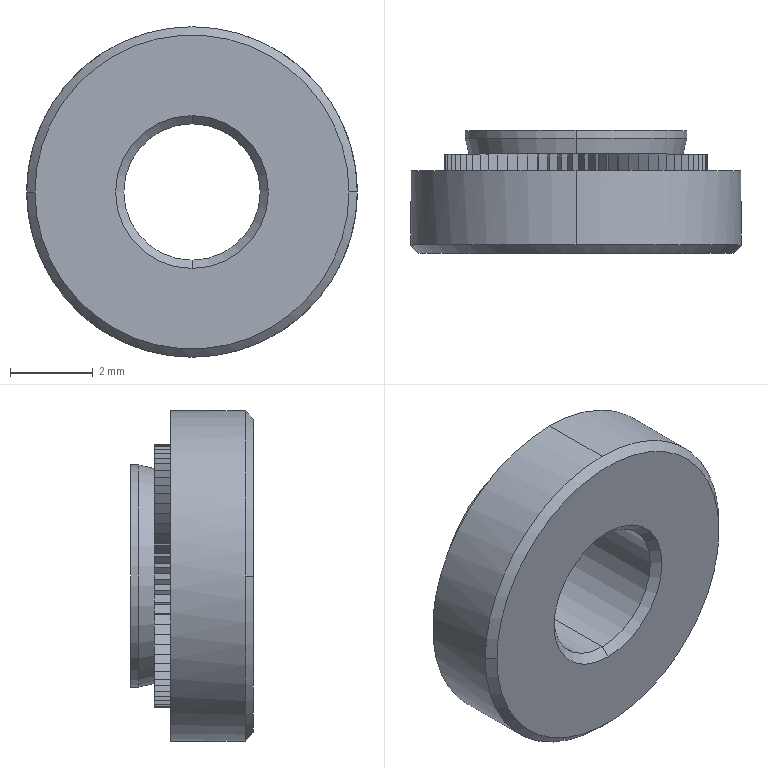Part | NX | features BREP 1 | 1 solid | 162 faces | box 8 x 2.97 x 8 mm | volume 98.301 mm3 | plane 148 | cone 8 | cylinder 6 | commonest cylinder face diameters 3.3 x2 5.38 x2 8 x2